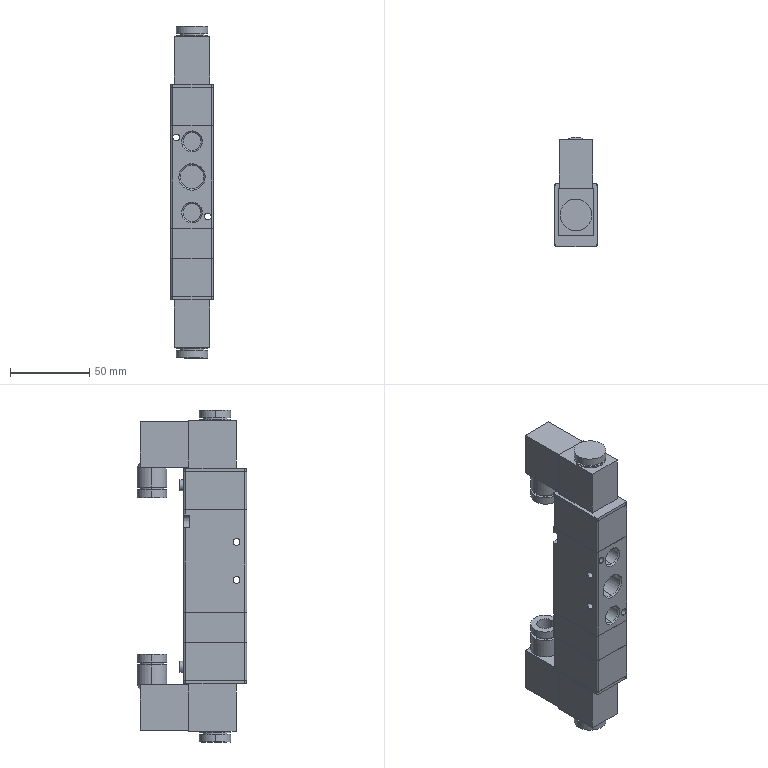Part | SolidWorks | features BaseBody 1 | 1 solid | 168 faces | box 27 x 69.3 x 209.8 mm | volume 222441 mm3 | cylinder 78 | plane 78 | cone 12 | commonest cylinder face diameters 2.4 x26 4.3 x8 15 x8 18.6 x8 20 x8 14.95 x6